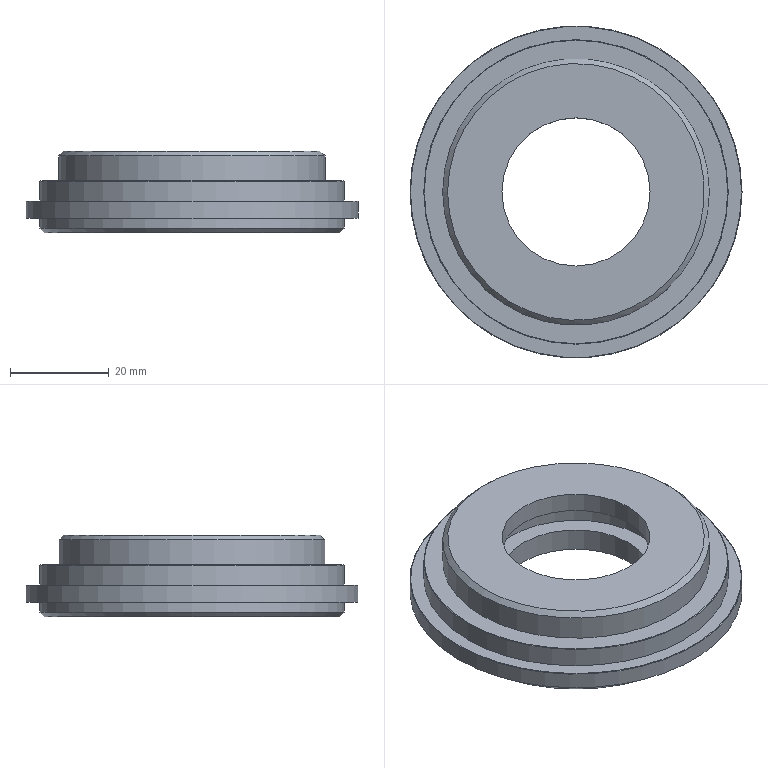Part | NX | features DATUM_CSYS 9, SKETCH 8, EXTRUDE 7, CHAMFER 6, DATUM_PLANE 3, Resize Face 2 | 1 solid | 20 faces | box 67.2 x 67.2 x 16.58 mm | volume 29560 mm3 | plane 8 | cylinder 8 | cone 4 | commonest cylinder face diameters 30 x2 61.62 x2 36.8 x1 51.34 x1 53.96 x1 67.2 x1
STEP:
#1=CARTESIAN_POINT('',(-25.98,0.,16.58));
#2=VERTEX_POINT('',#1);
#3=CARTESIAN_POINT('',(0.,0.,16.58));
#4=DIRECTION('',(0.,0.,-1.));
#5=DIRECTION('',(-1.,0.,0.));
#6=AXIS2_PLACEMENT_3D('',#3,#4,#5);
#7=CIRCLE('',#6,25.98);
#8=EDGE_CURVE('',#2,#2,#7,.F.);
#9=ORIENTED_EDGE('',*,*,#8,.T.);
#10=EDGE_LOOP('',(#9));
#11=FACE_BOUND('',#10,.T.);
#12=CARTESIAN_POINT('',(-15.,0.,16.58));
#13=VERTEX_POINT('',#12);
#14=CARTESIAN_POINT('',(0.,0.,16.58));
#15=DIRECTION('',(0.,0.,-1.));
#16=DIRECTION('',(-1.,0.,0.));
#17=AXIS2_PLACEMENT_3D('',#14,#15,#16);
#18=CIRCLE('',#17,15.);
#19=EDGE_CURVE('',#13,#13,#18,.T.);
#20=ORIENTED_EDGE('',*,*,#19,.T.);
#21=EDGE_LOOP('',(#20));
#22=FACE_BOUND('',#21,.T.);
#23=CARTESIAN_POINT('',(0.,0.,16.58));
#24=DIRECTION('',(0.,0.,-1.));
#25=DIRECTION('',(-1.,0.,0.));
#26=AXIS2_PLACEMENT_3D('',#23,#24,#25);
#27=PLANE('',#26);
#28=ADVANCED_FACE('',(#11,#22),#27,.F.);
#29=CARTESIAN_POINT('',(25.67,0.,2.98));
#30=VERTEX_POINT('',#29);
#31=CARTESIAN_POINT('',(0.,0.,2.98));
#32=DIRECTION('',(0.,0.,1.));
#33=DIRECTION('',(1.,0.,0.));
#34=AXIS2_PLACEMENT_3D('',#31,#32,#33);
#35=CIRCLE('',#34,25.67);
#36=EDGE_CURVE('',#30,#30,#35,.F.);
#37=ORIENTED_EDGE('',*,*,#36,.T.);
#38=EDGE_LOOP('',(#37));
#39=FACE_BOUND('',#38,.T.);
#40=CARTESIAN_POINT('',(15.,0.,2.98));
#41=VERTEX_POINT('',#40);
#42=CARTESIAN_POINT('',(0.,0.,2.98));
#43=DIRECTION('',(0.,0.,1.));
#44=DIRECTION('',(1.,0.,0.));
#45=AXIS2_PLACEMENT_3D('',#42,#43,#44);
#46=CIRCLE('',#45,15.);
#47=EDGE_CURVE('',#41,#41,#46,.T.);
#48=ORIENTED_EDGE('',*,*,#47,.T.);
#49=EDGE_LOOP('',(#48));
#50=FACE_BOUND('',#49,.T.);
#51=CARTESIAN_POINT('',(0.,0.,2.98));
#52=DIRECTION('',(0.,0.,1.));
#53=DIRECTION('',(1.,0.,0.));
#54=AXIS2_PLACEMENT_3D('',#51,#52,#53);
#55=PLANE('',#54);
#56=ADVANCED_FACE('',(#39,#50),#55,.F.);
#57=CARTESIAN_POINT('',(-33.6,0.,6.36));
#58=VERTEX_POINT('',#57);
#59=CARTESIAN_POINT('',(0.,0.,6.36));
#60=DIRECTION('',(0.,0.,-1.));
#61=DIRECTION('',(-1.,0.,0.));
#62=AXIS2_PLACEMENT_3D('',#59,#60,#61);
#63=CIRCLE('',#62,33.6);
#64=EDGE_CURVE('',#58,#58,#63,.T.);
#65=ORIENTED_EDGE('',*,*,#64,.T.);
#66=EDGE_LOOP('',(#65));
#67=FACE_BOUND('',#66,.T.);
#68=CARTESIAN_POINT('',(33.6,0.,2.98));
#69=VERTEX_POINT('',#68);
#70=CARTESIAN_POINT('',(0.,0.,2.98));
#71=DIRECTION('',(0.,0.,1.));
#72=DIRECTION('',(1.,0.,0.));
#73=AXIS2_PLACEMENT_3D('',#70,#71,#72);
#74=CIRCLE('',#73,33.6);
#75=EDGE_CURVE('',#69,#69,#74,.T.);
#76=ORIENTED_EDGE('',*,*,#75,.T.);
#77=EDGE_LOOP('',(#76));
#78=FACE_BOUND('',#77,.T.);
#79=CARTESIAN_POINT('',(0.,0.,16.58));
#80=DIRECTION('',(0.,0.,-1.));
#81=DIRECTION('',(-1.,0.,0.));
#82=AXIS2_PLACEMENT_3D('',#79,#80,#81);
#83=CYLINDRICAL_SURFACE('',#82,33.6);
#84=ADVANCED_FACE('',(#67,#78),#83,.T.);
#85=CARTESIAN_POINT('',(-29.81,0.,0.));
#86=VERTEX_POINT('',#85);
#87=CARTESIAN_POINT('',(0.,0.,0.));
#88=DIRECTION('',(0.,0.,-1.));
#89=DIRECTION('',(-1.,0.,0.));
#90=AXIS2_PLACEMENT_3D('',#87,#88,#89);
#91=CIRCLE('',#90,29.81);
#92=EDGE_CURVE('',#86,#86,#91,.T.);
#93=ORIENTED_EDGE('',*,*,#92,.T.);
#94=EDGE_LOOP('',(#93));
#95=FACE_BOUND('',#94,.T.);
#96=CARTESIAN_POINT('',(25.67,0.,0.));
#97=VERTEX_POINT('',#96);
#98=CARTESIAN_POINT('',(0.,0.,0.));
#99=DIRECTION('',(0.,0.,1.));
#100=DIRECTION('',(1.,0.,0.));
#101=AXIS2_PLACEMENT_3D('',#98,#99,#100);
#102=CIRCLE('',#101,25.67);
#103=EDGE_CURVE('',#97,#97,#102,.T.);
#104=ORIENTED_EDGE('',*,*,#103,.T.);
#105=EDGE_LOOP('',(#104));
#106=FACE_BOUND('',#105,.T.);
#107=CARTESIAN_POINT('',(0.,0.,0.));
#108=DIRECTION('',(0.,0.,-1.));
#109=DIRECTION('',(-1.,0.,0.));
#110=AXIS2_PLACEMENT_3D('',#107,#108,#109);
#111=PLANE('',#110);
#112=ADVANCED_FACE('',(#95,#106),#111,.T.);
#113=ORIENTED_EDGE('',*,*,#47,.F.);
#114=EDGE_LOOP('',(#113));
#115=FACE_BOUND('',#114,.T.);
#116=CARTESIAN_POINT('',(15.,0.,7.74));
#117=VERTEX_POINT('',#116);
#118=CARTESIAN_POINT('',(0.,0.,7.74));
#119=DIRECTION('',(0.,0.,1.));
#120=DIRECTION('',(1.,0.,0.));
#121=AXIS2_PLACEMENT_3D('',#118,#119,#120);
#122=CIRCLE('',#121,15.);
#123=EDGE_CURVE('',#117,#117,#122,.T.);
#124=ORIENTED_EDGE('',*,*,#123,.T.);
#125=EDGE_LOOP('',(#124));
#126=FACE_BOUND('',#125,.T.);
#127=CARTESIAN_POINT('',(0.,0.,-1.658));
#128=DIRECTION('',(0.,0.,1.));
#129=DIRECTION('',(1.,0.,0.));
#130=AXIS2_PLACEMENT_3D('',#127,#128,#129);
#131=CYLINDRICAL_SURFACE('',#130,15.);
#132=ADVANCED_FACE('',(#115,#126),#131,.F.);
#133=ORIENTED_EDGE('',*,*,#19,.F.);
#134=EDGE_LOOP('',(#133));
#135=FACE_BOUND('',#134,.T.);
#136=CARTESIAN_POINT('',(15.,0.,12.58));
#137=VERTEX_POINT('',#136);
#138=CARTESIAN_POINT('',(0.,0.,12.58));
#139=DIRECTION('',(0.,0.,1.));
#140=DIRECTION('',(1.,0.,0.));
#141=AXIS2_PLACEMENT_3D('',#138,#139,#140);
#142=CIRCLE('',#141,15.);
#143=EDGE_CURVE('',#137,#137,#142,.T.);
#144=ORIENTED_EDGE('',*,*,#143,.F.);
#145=EDGE_LOOP('',(#144));
#146=FACE_BOUND('',#145,.T.);
#147=CARTESIAN_POINT('',(0.,0.,-1.658));
#148=DIRECTION('',(0.,0.,1.));
#149=DIRECTION('',(1.,0.,0.));
#150=AXIS2_PLACEMENT_3D('',#147,#148,#149);
#151=CYLINDRICAL_SURFACE('',#150,15.);
#152=ADVANCED_FACE('',(#135,#146),#151,.F.);
#153=CARTESIAN_POINT('',(18.4,0.,7.74));
#154=VERTEX_POINT('',#153);
#155=CARTESIAN_POINT('',(0.,0.,7.74));
#156=DIRECTION('',(0.,0.,1.));
#157=DIRECTION('',(1.,0.,0.));
#158=AXIS2_PLACEMENT_3D('',#155,#156,#157);
#159=CIRCLE('',#158,18.4);
#160=EDGE_CURVE('',#154,#154,#159,.F.);
#161=ORIENTED_EDGE('',*,*,#160,.T.);
#162=EDGE_LOOP('',(#161));
#163=FACE_BOUND('',#162,.T.);
#164=CARTESIAN_POINT('',(18.4,0.,12.58));
#165=VERTEX_POINT('',#164);
#166=CARTESIAN_POINT('',(0.,0.,12.58));
#167=DIRECTION('',(0.,0.,1.));
#168=DIRECTION('',(1.,0.,0.));
#169=AXIS2_PLACEMENT_3D('',#166,#167,#168);
#170=CIRCLE('',#169,18.4);
#171=EDGE_CURVE('',#165,#165,#170,.F.);
#172=ORIENTED_EDGE('',*,*,#171,.F.);
#173=EDGE_LOOP('',(#172));
#174=FACE_BOUND('',#173,.T.);
#175=CARTESIAN_POINT('',(0.,0.,7.74));
#176=DIRECTION('',(0.,0.,1.));
#177=DIRECTION('',(1.,0.,0.));
#178=AXIS2_PLACEMENT_3D('',#175,#176,#177);
#179=CYLINDRICAL_SURFACE('',#178,18.4);
#180=ADVANCED_FACE('',(#163,#174),#179,.F.);
#181=ORIENTED_EDGE('',*,*,#123,.F.);
#182=EDGE_LOOP('',(#181));
#183=FACE_BOUND('',#182,.T.);
#184=ORIENTED_EDGE('',*,*,#160,.F.);
#185=EDGE_LOOP('',(#184));
#186=FACE_BOUND('',#185,.T.);
#187=CARTESIAN_POINT('',(0.,0.,7.74));
#188=DIRECTION('',(0.,0.,1.));
#189=DIRECTION('',(1.,0.,0.));
#190=AXIS2_PLACEMENT_3D('',#187,#188,#189);
#191=PLANE('',#190);
#192=ADVANCED_FACE('',(#183,#186),#191,.T.);
#193=ORIENTED_EDGE('',*,*,#143,.T.);
#194=EDGE_LOOP('',(#193));
#195=FACE_BOUND('',#194,.T.);
#196=ORIENTED_EDGE('',*,*,#171,.T.);
#197=EDGE_LOOP('',(#196));
#198=FACE_BOUND('',#197,.T.);
#199=CARTESIAN_POINT('',(0.,0.,12.58));
#200=DIRECTION('',(0.,0.,1.));
#201=DIRECTION('',(1.,0.,0.));
#202=AXIS2_PLACEMENT_3D('',#199,#200,#201);
#203=PLANE('',#202);
#204=ADVANCED_FACE('',(#195,#198),#203,.F.);
#205=CARTESIAN_POINT('',(-30.81,0.,10.5));
#206=VERTEX_POINT('',#205);
#207=CARTESIAN_POINT('',(0.,0.,10.5));
#208=DIRECTION('',(0.,0.,-1.));
#209=DIRECTION('',(-1.,0.,0.));
#210=AXIS2_PLACEMENT_3D('',#207,#208,#209);
#211=CIRCLE('',#210,30.81);
#212=EDGE_CURVE('',#206,#206,#211,.T.);
#213=ORIENTED_EDGE('',*,*,#212,.T.);
#214=EDGE_LOOP('',(#213));
#215=FACE_BOUND('',#214,.T.);
#216=CARTESIAN_POINT('',(30.81,0.,6.46));
#217=VERTEX_POINT('',#216);
#218=CARTESIAN_POINT('',(0.,0.,6.46));
#219=DIRECTION('',(0.,0.,-1.));
#220=DIRECTION('',(1.,0.,0.));
#221=AXIS2_PLACEMENT_3D('',#218,#219,#220);
#222=CIRCLE('',#221,30.81);
#223=EDGE_CURVE('',#217,#217,#222,.F.);
#224=ORIENTED_EDGE('',*,*,#223,.T.);
#225=EDGE_LOOP('',(#224));
#226=FACE_BOUND('',#225,.T.);
#227=CARTESIAN_POINT('',(0.,0.,6.46));
#228=DIRECTION('',(0.,0.,1.));
#229=DIRECTION('',(1.,0.,0.));
#230=AXIS2_PLACEMENT_3D('',#227,#228,#229);
#231=CYLINDRICAL_SURFACE('',#230,30.81);
#232=ADVANCED_FACE('',(#215,#226),#231,.T.);
#233=CARTESIAN_POINT('',(-33.5,0.,6.46));
#234=VERTEX_POINT('',#233);
#235=CARTESIAN_POINT('',(0.,0.,6.46));
#236=DIRECTION('',(0.,0.,-1.));
#237=DIRECTION('',(-1.,0.,0.));
#238=AXIS2_PLACEMENT_3D('',#235,#236,#237);
#239=CIRCLE('',#238,33.5);
#240=EDGE_CURVE('',#234,#234,#239,.F.);
#241=ORIENTED_EDGE('',*,*,#240,.T.);
#242=EDGE_LOOP('',(#241));
#243=FACE_BOUND('',#242,.T.);
#244=ORIENTED_EDGE('',*,*,#223,.F.);
#245=EDGE_LOOP('',(#244));
#246=FACE_BOUND('',#245,.T.);
#247=CARTESIAN_POINT('',(0.,0.,6.46));
#248=DIRECTION('',(0.,0.,-1.));
#249=DIRECTION('',(-1.,0.,0.));
#250=AXIS2_PLACEMENT_3D('',#247,#248,#249);
#251=PLANE('',#250);
#252=ADVANCED_FACE('',(#243,#246),#251,.F.);
#253=CARTESIAN_POINT('',(-26.98,0.,15.58));
#254=VERTEX_POINT('',#253);
#255=CARTESIAN_POINT('',(0.,0.,15.58));
#256=DIRECTION('',(0.,0.,-1.));
#257=DIRECTION('',(-1.,0.,0.));
#258=AXIS2_PLACEMENT_3D('',#255,#256,#257);
#259=CIRCLE('',#258,26.98);
#260=EDGE_CURVE('',#254,#254,#259,.T.);
#261=ORIENTED_EDGE('',*,*,#260,.T.);
#262=EDGE_LOOP('',(#261));
#263=FACE_BOUND('',#262,.T.);
#264=CARTESIAN_POINT('',(26.98,0.,10.6));
#265=VERTEX_POINT('',#264);
#266=CARTESIAN_POINT('',(0.,0.,10.6));
#267=DIRECTION('',(0.,0.,-1.));
#268=DIRECTION('',(1.,0.,0.));
#269=AXIS2_PLACEMENT_3D('',#266,#267,#268);
#270=CIRCLE('',#269,26.98);
#271=EDGE_CURVE('',#265,#265,#270,.F.);
#272=ORIENTED_EDGE('',*,*,#271,.T.);
#273=EDGE_LOOP('',(#272));
#274=FACE_BOUND('',#273,.T.);
#275=CARTESIAN_POINT('',(0.,0.,10.6));
#276=DIRECTION('',(0.,0.,1.));
#277=DIRECTION('',(1.,0.,0.));
#278=AXIS2_PLACEMENT_3D('',#275,#276,#277);
#279=CYLINDRICAL_SURFACE('',#278,26.98);
#280=ADVANCED_FACE('',(#263,#274),#279,.T.);
#281=CARTESIAN_POINT('',(-30.71,0.,10.6));
#282=VERTEX_POINT('',#281);
#283=CARTESIAN_POINT('',(0.,0.,10.6));
#284=DIRECTION('',(0.,0.,-1.));
#285=DIRECTION('',(-1.,0.,0.));
#286=AXIS2_PLACEMENT_3D('',#283,#284,#285);
#287=CIRCLE('',#286,30.71);
#288=EDGE_CURVE('',#282,#282,#287,.F.);
#289=ORIENTED_EDGE('',*,*,#288,.T.);
#290=EDGE_LOOP('',(#289));
#291=FACE_BOUND('',#290,.T.);
#292=ORIENTED_EDGE('',*,*,#271,.F.);
#293=EDGE_LOOP('',(#292));
#294=FACE_BOUND('',#293,.T.);
#295=CARTESIAN_POINT('',(0.,0.,10.6));
#296=DIRECTION('',(0.,0.,-1.));
#297=DIRECTION('',(-1.,0.,0.));
#298=AXIS2_PLACEMENT_3D('',#295,#296,#297);
#299=PLANE('',#298);
#300=ADVANCED_FACE('',(#291,#294),#299,.F.);
#301=CARTESIAN_POINT('',(-30.81,0.,1.));
#302=VERTEX_POINT('',#301);
#303=CARTESIAN_POINT('',(0.,0.,1.));
#304=DIRECTION('',(0.,0.,-1.));
#305=DIRECTION('',(-1.,0.,0.));
#306=AXIS2_PLACEMENT_3D('',#303,#304,#305);
#307=CIRCLE('',#306,30.81);
#308=EDGE_CURVE('',#302,#302,#307,.F.);
#309=ORIENTED_EDGE('',*,*,#308,.T.);
#310=EDGE_LOOP('',(#309));
#311=FACE_BOUND('',#310,.T.);
#312=CARTESIAN_POINT('',(30.81,0.,2.98));
#313=VERTEX_POINT('',#312);
#314=CARTESIAN_POINT('',(0.,0.,2.98));
#315=DIRECTION('',(0.,0.,1.));
#316=DIRECTION('',(1.,0.,0.));
#317=AXIS2_PLACEMENT_3D('',#314,#315,#316);
#318=CIRCLE('',#317,30.81);
#319=EDGE_CURVE('',#313,#313,#318,.F.);
#320=ORIENTED_EDGE('',*,*,#319,.T.);
#321=EDGE_LOOP('',(#320));
#322=FACE_BOUND('',#321,.T.);
#323=CARTESIAN_POINT('',(0.,0.,2.98));
#324=DIRECTION('',(0.,0.,-1.));
#325=DIRECTION('',(-1.,0.,0.));
#326=AXIS2_PLACEMENT_3D('',#323,#324,#325);
#327=CYLINDRICAL_SURFACE('',#326,30.81);
#328=ADVANCED_FACE('',(#311,#322),#327,.T.);
#329=ORIENTED_EDGE('',*,*,#75,.F.);
#330=EDGE_LOOP('',(#329));
#331=FACE_BOUND('',#330,.T.);
#332=ORIENTED_EDGE('',*,*,#319,.F.);
#333=EDGE_LOOP('',(#332));
#334=FACE_BOUND('',#333,.T.);
#335=CARTESIAN_POINT('',(0.,0.,2.98));
#336=DIRECTION('',(0.,0.,1.));
#337=DIRECTION('',(1.,0.,0.));
#338=AXIS2_PLACEMENT_3D('',#335,#336,#337);
#339=PLANE('',#338);
#340=ADVANCED_FACE('',(#331,#334),#339,.F.);
#341=ORIENTED_EDGE('',*,*,#36,.F.);
#342=EDGE_LOOP('',(#341));
#343=FACE_BOUND('',#342,.T.);
#344=ORIENTED_EDGE('',*,*,#103,.F.);
#345=EDGE_LOOP('',(#344));
#346=FACE_BOUND('',#345,.T.);
#347=CARTESIAN_POINT('',(0.,0.,2.98));
#348=DIRECTION('',(0.,0.,-1.));
#349=DIRECTION('',(-1.,0.,0.));
#350=AXIS2_PLACEMENT_3D('',#347,#348,#349);
#351=CYLINDRICAL_SURFACE('',#350,25.67);
#352=ADVANCED_FACE('',(#343,#346),#351,.F.);
#353=ORIENTED_EDGE('',*,*,#288,.F.);
#354=EDGE_LOOP('',(#353));
#355=FACE_BOUND('',#354,.T.);
#356=ORIENTED_EDGE('',*,*,#212,.F.);
#357=EDGE_LOOP('',(#356));
#358=FACE_BOUND('',#357,.T.);
#359=CARTESIAN_POINT('',(0.,0.,10.5));
#360=DIRECTION('',(0.,0.,-1.));
#361=DIRECTION('',(-1.,0.,0.));
#362=AXIS2_PLACEMENT_3D('',#359,#360,#361);
#363=CONICAL_SURFACE('',#362,30.81,0.7854);
#364=ADVANCED_FACE('',(#355,#358),#363,.T.);
#365=ORIENTED_EDGE('',*,*,#240,.F.);
#366=EDGE_LOOP('',(#365));
#367=FACE_BOUND('',#366,.T.);
#368=ORIENTED_EDGE('',*,*,#64,.F.);
#369=EDGE_LOOP('',(#368));
#370=FACE_BOUND('',#369,.T.);
#371=CARTESIAN_POINT('',(0.,0.,6.36));
#372=DIRECTION('',(0.,0.,-1.));
#373=DIRECTION('',(-1.,0.,0.));
#374=AXIS2_PLACEMENT_3D('',#371,#372,#373);
#375=CONICAL_SURFACE('',#374,33.6,0.7854);
#376=ADVANCED_FACE('',(#367,#370),#375,.T.);
#377=ORIENTED_EDGE('',*,*,#92,.F.);
#378=EDGE_LOOP('',(#377));
#379=FACE_BOUND('',#378,.T.);
#380=ORIENTED_EDGE('',*,*,#308,.F.);
#381=EDGE_LOOP('',(#380));
#382=FACE_BOUND('',#381,.T.);
#383=CARTESIAN_POINT('',(0.,0.,1.));
#384=DIRECTION('',(0.,0.,1.));
#385=DIRECTION('',(1.,0.,0.));
#386=AXIS2_PLACEMENT_3D('',#383,#384,#385);
#387=CONICAL_SURFACE('',#386,30.81,0.7854);
#388=ADVANCED_FACE('',(#379,#382),#387,.T.);
#389=ORIENTED_EDGE('',*,*,#8,.F.);
#390=EDGE_LOOP('',(#389));
#391=FACE_BOUND('',#390,.T.);
#392=ORIENTED_EDGE('',*,*,#260,.F.);
#393=EDGE_LOOP('',(#392));
#394=FACE_BOUND('',#393,.T.);
#395=CARTESIAN_POINT('',(0.,0.,15.58));
#396=DIRECTION('',(0.,0.,-1.));
#397=DIRECTION('',(-1.,0.,0.));
#398=AXIS2_PLACEMENT_3D('',#395,#396,#397);
#399=CONICAL_SURFACE('',#398,26.98,0.7854);
#400=ADVANCED_FACE('',(#391,#394),#399,.T.);
#401=CLOSED_SHELL('',(#28,#56,#84,#112,#132,#152,#180,#192,#204,#232,#252,#280,#300,#328,#340,#352,#364,#376,#388,#400));
#402=MANIFOLD_SOLID_BREP('',#401);
#403=(LENGTH_UNIT()NAMED_UNIT(*)SI_UNIT(.MILLI.,.METRE.));
#404=UNCERTAINTY_MEASURE_WITH_UNIT(LENGTH_MEASURE(0.00001),#403,'','');
#405=(NAMED_UNIT(*)PLANE_ANGLE_UNIT()SI_UNIT($,.RADIAN.));
#406=(NAMED_UNIT(*)SI_UNIT($,.STERADIAN.)SOLID_ANGLE_UNIT());
#407=(GEOMETRIC_REPRESENTATION_CONTEXT(3)GLOBAL_UNCERTAINTY_ASSIGNED_CONTEXT((#404))GLOBAL_UNIT_ASSIGNED_CONTEXT((#403,#405,#406))REPRESENTATION_CONTEXT('',''));
#408=ADVANCED_BREP_SHAPE_REPRESENTATION('',(#402),#407);